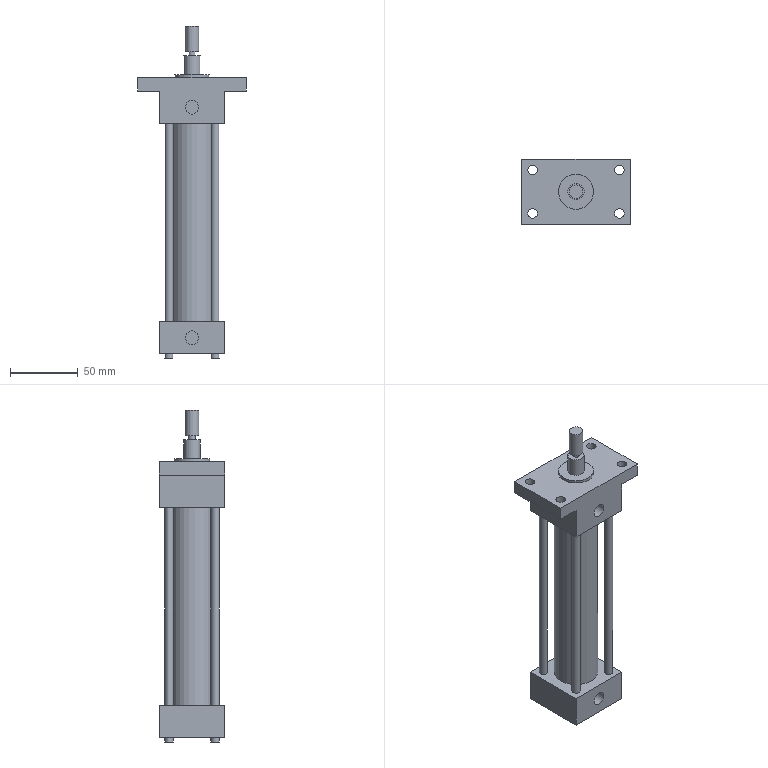Part | NX | features solid 2 | 1 solid | 48 faces | box 80 x 48 x 245 mm | volume 201071 mm3 | plane 28 | cylinder 20 | commonest cylinder face diameters 6 x8 7 x4 10 x3 5 x1 12 x1 26 x1
STEP:
#1=CARTESIAN_POINT('',(560.,11.,-204.));
#2=VERTEX_POINT('',#1);
#3=CARTESIAN_POINT('',(560.,-5.,-204.));
#4=DIRECTION('',(0.,0.,1.));
#5=DIRECTION('',(0.,1.,0.));
#6=AXIS2_PLACEMENT_3D('',#3,#4,#5);
#7=CIRCLE('',#6,16.);
#8=EDGE_CURVE('',#2,#2,#7,.T.);
#9=ORIENTED_EDGE('',*,*,#8,.F.);
#10=EDGE_LOOP('',(#9));
#11=FACE_BOUND('',#10,.T.);
#12=CARTESIAN_POINT('',(560.,11.,-350.));
#13=VERTEX_POINT('',#12);
#14=CARTESIAN_POINT('',(560.,-5.,-350.));
#15=DIRECTION('',(0.,0.,1.));
#16=DIRECTION('',(0.,1.,0.));
#17=AXIS2_PLACEMENT_3D('',#14,#15,#16);
#18=CIRCLE('',#17,16.);
#19=EDGE_CURVE('',#13,#13,#18,.F.);
#20=ORIENTED_EDGE('',*,*,#19,.F.);
#21=EDGE_LOOP('',(#20));
#22=FACE_BOUND('',#21,.T.);
#23=CARTESIAN_POINT('',(560.,-5.,-374.));
#24=DIRECTION('',(0.,0.,1.));
#25=DIRECTION('',(0.,-1.,0.));
#26=AXIS2_PLACEMENT_3D('',#23,#24,#25);
#27=CYLINDRICAL_SURFACE('',#26,16.);
#28=ADVANCED_FACE('',(#11,#22),#27,.T.);
#29=CARTESIAN_POINT('',(560.,-11.,-154.));
#30=VERTEX_POINT('',#29);
#31=CARTESIAN_POINT('',(560.,-5.,-154.));
#32=DIRECTION('',(0.,0.,-1.));
#33=DIRECTION('',(0.,-1.,0.));
#34=AXIS2_PLACEMENT_3D('',#31,#32,#33);
#35=CIRCLE('',#34,6.);
#36=EDGE_CURVE('',#30,#30,#35,.T.);
#37=ORIENTED_EDGE('',*,*,#36,.F.);
#38=EDGE_LOOP('',(#37));
#39=FACE_BOUND('',#38,.T.);
#40=CARTESIAN_POINT('',(560.,-7.5,-154.));
#41=VERTEX_POINT('',#40);
#42=CARTESIAN_POINT('',(560.,-5.,-154.));
#43=DIRECTION('',(0.,0.,-1.));
#44=DIRECTION('',(0.,-1.,0.));
#45=AXIS2_PLACEMENT_3D('',#42,#43,#44);
#46=CIRCLE('',#45,2.5);
#47=EDGE_CURVE('',#41,#41,#46,.T.);
#48=ORIENTED_EDGE('',*,*,#47,.T.);
#49=EDGE_LOOP('',(#48));
#50=FACE_BOUND('',#49,.T.);
#51=CARTESIAN_POINT('',(560.,-5.,-154.));
#52=DIRECTION('',(0.,0.,1.));
#53=DIRECTION('',(0.,-1.,0.));
#54=AXIS2_PLACEMENT_3D('',#51,#52,#53);
#55=PLANE('',#54);
#56=ADVANCED_FACE('',(#39,#50),#55,.T.);
#57=CARTESIAN_POINT('',(560.,-18.,-168.));
#58=VERTEX_POINT('',#57);
#59=CARTESIAN_POINT('',(560.,-5.,-168.));
#60=DIRECTION('',(0.,0.,-1.));
#61=DIRECTION('',(0.,-1.,0.));
#62=AXIS2_PLACEMENT_3D('',#59,#60,#61);
#63=CIRCLE('',#62,13.);
#64=EDGE_CURVE('',#58,#58,#63,.T.);
#65=ORIENTED_EDGE('',*,*,#64,.F.);
#66=EDGE_LOOP('',(#65));
#67=FACE_BOUND('',#66,.T.);
#68=CARTESIAN_POINT('',(560.,-11.,-168.));
#69=VERTEX_POINT('',#68);
#70=CARTESIAN_POINT('',(560.,-5.,-168.));
#71=DIRECTION('',(0.,0.,-1.));
#72=DIRECTION('',(0.,-1.,0.));
#73=AXIS2_PLACEMENT_3D('',#70,#71,#72);
#74=CIRCLE('',#73,6.);
#75=EDGE_CURVE('',#69,#69,#74,.F.);
#76=ORIENTED_EDGE('',*,*,#75,.F.);
#77=EDGE_LOOP('',(#76));
#78=FACE_BOUND('',#77,.T.);
#79=CARTESIAN_POINT('',(560.,-5.,-168.));
#80=DIRECTION('',(0.,0.,1.));
#81=DIRECTION('',(0.,-1.,0.));
#82=AXIS2_PLACEMENT_3D('',#79,#80,#81);
#83=PLANE('',#82);
#84=ADVANCED_FACE('',(#67,#78),#83,.T.);
#85=CARTESIAN_POINT('',(528.,7.5,-170.));
#86=VERTEX_POINT('',#85);
#87=CARTESIAN_POINT('',(528.,11.,-170.));
#88=DIRECTION('',(0.,0.,-1.));
#89=DIRECTION('',(0.,-1.,0.));
#90=AXIS2_PLACEMENT_3D('',#87,#88,#89);
#91=CIRCLE('',#90,3.5);
#92=EDGE_CURVE('',#86,#86,#91,.T.);
#93=ORIENTED_EDGE('',*,*,#92,.T.);
#94=EDGE_LOOP('',(#93));
#95=FACE_BOUND('',#94,.T.);
#96=CARTESIAN_POINT('',(592.,-24.5,-170.));
#97=VERTEX_POINT('',#96);
#98=CARTESIAN_POINT('',(592.,-21.,-170.));
#99=DIRECTION('',(0.,0.,-1.));
#100=DIRECTION('',(0.,-1.,0.));
#101=AXIS2_PLACEMENT_3D('',#98,#99,#100);
#102=CIRCLE('',#101,3.5);
#103=EDGE_CURVE('',#97,#97,#102,.T.);
#104=ORIENTED_EDGE('',*,*,#103,.T.);
#105=EDGE_LOOP('',(#104));
#106=FACE_BOUND('',#105,.T.);
#107=CARTESIAN_POINT('',(520.,19.,-170.));
#108=VERTEX_POINT('',#107);
#109=CARTESIAN_POINT('',(520.,-29.,-170.));
#110=VERTEX_POINT('',#109);
#111=CARTESIAN_POINT('',(520.,19.,-170.));
#112=DIRECTION('',(0.,-1.,0.));
#113=VECTOR('',#112,1000.);
#114=LINE('',#111,#113);
#115=EDGE_CURVE('',#108,#110,#114,.T.);
#116=ORIENTED_EDGE('',*,*,#115,.T.);
#117=CARTESIAN_POINT('',(600.,-29.,-170.));
#118=VERTEX_POINT('',#117);
#119=CARTESIAN_POINT('',(600.,-29.,-170.));
#120=DIRECTION('',(-1.,0.,0.));
#121=VECTOR('',#120,1000.);
#122=LINE('',#119,#121);
#123=EDGE_CURVE('',#118,#110,#122,.T.);
#124=ORIENTED_EDGE('',*,*,#123,.F.);
#125=CARTESIAN_POINT('',(600.,19.,-170.));
#126=VERTEX_POINT('',#125);
#127=CARTESIAN_POINT('',(600.,19.,-170.));
#128=DIRECTION('',(0.,-1.,0.));
#129=VECTOR('',#128,1000.);
#130=LINE('',#127,#129);
#131=EDGE_CURVE('',#126,#118,#130,.T.);
#132=ORIENTED_EDGE('',*,*,#131,.F.);
#133=CARTESIAN_POINT('',(536.,19.,-170.));
#134=DIRECTION('',(-1.,0.,0.));
#135=VECTOR('',#134,1000.);
#136=LINE('',#133,#135);
#137=EDGE_CURVE('',#126,#108,#136,.T.);
#138=ORIENTED_EDGE('',*,*,#137,.T.);
#139=EDGE_LOOP('',(#116,#124,#132,#138));
#140=FACE_BOUND('',#139,.T.);
#141=CARTESIAN_POINT('',(592.,7.5,-170.));
#142=VERTEX_POINT('',#141);
#143=CARTESIAN_POINT('',(592.,11.,-170.));
#144=DIRECTION('',(0.,0.,-1.));
#145=DIRECTION('',(0.,-1.,0.));
#146=AXIS2_PLACEMENT_3D('',#143,#144,#145);
#147=CIRCLE('',#146,3.5);
#148=EDGE_CURVE('',#142,#142,#147,.T.);
#149=ORIENTED_EDGE('',*,*,#148,.T.);
#150=EDGE_LOOP('',(#149));
#151=FACE_BOUND('',#150,.T.);
#152=CARTESIAN_POINT('',(528.,-24.5,-170.));
#153=VERTEX_POINT('',#152);
#154=CARTESIAN_POINT('',(528.,-21.,-170.));
#155=DIRECTION('',(0.,0.,-1.));
#156=DIRECTION('',(0.,-1.,0.));
#157=AXIS2_PLACEMENT_3D('',#154,#155,#156);
#158=CIRCLE('',#157,3.5);
#159=EDGE_CURVE('',#153,#153,#158,.T.);
#160=ORIENTED_EDGE('',*,*,#159,.T.);
#161=EDGE_LOOP('',(#160));
#162=FACE_BOUND('',#161,.T.);
#163=CARTESIAN_POINT('',(560.,8.,-170.));
#164=VERTEX_POINT('',#163);
#165=CARTESIAN_POINT('',(560.,-5.,-170.));
#166=DIRECTION('',(0.,0.,1.));
#167=DIRECTION('',(0.,1.,0.));
#168=AXIS2_PLACEMENT_3D('',#165,#166,#167);
#169=CIRCLE('',#168,13.);
#170=EDGE_CURVE('',#164,#164,#169,.F.);
#171=ORIENTED_EDGE('',*,*,#170,.T.);
#172=EDGE_LOOP('',(#171));
#173=FACE_BOUND('',#172,.T.);
#174=CARTESIAN_POINT('',(520.,-29.,-170.));
#175=DIRECTION('',(0.,0.,-1.));
#176=DIRECTION('',(0.,1.,0.));
#177=AXIS2_PLACEMENT_3D('',#174,#175,#176);
#178=PLANE('',#177);
#179=ADVANCED_FACE('',(#95,#106,#140,#151,#162,#173),#178,.F.);
#180=CARTESIAN_POINT('',(584.,-29.,-180.));
#181=VERTEX_POINT('',#180);
#182=CARTESIAN_POINT('',(584.,19.,-180.));
#183=VERTEX_POINT('',#182);
#184=CARTESIAN_POINT('',(584.,-29.,-180.));
#185=DIRECTION('',(0.,1.,0.));
#186=VECTOR('',#185,1000.);
#187=LINE('',#184,#186);
#188=EDGE_CURVE('',#181,#183,#187,.T.);
#189=ORIENTED_EDGE('',*,*,#188,.T.);
#190=CARTESIAN_POINT('',(600.,19.,-180.));
#191=VERTEX_POINT('',#190);
#192=CARTESIAN_POINT('',(536.,19.,-180.));
#193=DIRECTION('',(-1.,0.,0.));
#194=VECTOR('',#193,1000.);
#195=LINE('',#192,#194);
#196=EDGE_CURVE('',#191,#183,#195,.T.);
#197=ORIENTED_EDGE('',*,*,#196,.F.);
#198=CARTESIAN_POINT('',(600.,-29.,-180.));
#199=VERTEX_POINT('',#198);
#200=CARTESIAN_POINT('',(600.,19.,-180.));
#201=DIRECTION('',(0.,-1.,0.));
#202=VECTOR('',#201,1000.);
#203=LINE('',#200,#202);
#204=EDGE_CURVE('',#191,#199,#203,.T.);
#205=ORIENTED_EDGE('',*,*,#204,.T.);
#206=CARTESIAN_POINT('',(600.,-29.,-180.));
#207=DIRECTION('',(-1.,0.,0.));
#208=VECTOR('',#207,1000.);
#209=LINE('',#206,#208);
#210=EDGE_CURVE('',#199,#181,#209,.T.);
#211=ORIENTED_EDGE('',*,*,#210,.T.);
#212=EDGE_LOOP('',(#189,#197,#205,#211));
#213=FACE_BOUND('',#212,.T.);
#214=CARTESIAN_POINT('',(592.,-24.5,-180.));
#215=VERTEX_POINT('',#214);
#216=CARTESIAN_POINT('',(592.,-21.,-180.));
#217=DIRECTION('',(0.,0.,-1.));
#218=DIRECTION('',(0.,-1.,0.));
#219=AXIS2_PLACEMENT_3D('',#216,#217,#218);
#220=CIRCLE('',#219,3.5);
#221=EDGE_CURVE('',#215,#215,#220,.T.);
#222=ORIENTED_EDGE('',*,*,#221,.F.);
#223=EDGE_LOOP('',(#222));
#224=FACE_BOUND('',#223,.T.);
#225=CARTESIAN_POINT('',(592.,7.5,-180.));
#226=VERTEX_POINT('',#225);
#227=CARTESIAN_POINT('',(592.,11.,-180.));
#228=DIRECTION('',(0.,0.,-1.));
#229=DIRECTION('',(0.,-1.,0.));
#230=AXIS2_PLACEMENT_3D('',#227,#228,#229);
#231=CIRCLE('',#230,3.5);
#232=EDGE_CURVE('',#226,#226,#231,.T.);
#233=ORIENTED_EDGE('',*,*,#232,.F.);
#234=EDGE_LOOP('',(#233));
#235=FACE_BOUND('',#234,.T.);
#236=CARTESIAN_POINT('',(520.,-29.,-180.));
#237=DIRECTION('',(0.,0.,-1.));
#238=DIRECTION('',(0.,1.,0.));
#239=AXIS2_PLACEMENT_3D('',#236,#237,#238);
#240=PLANE('',#239);
#241=ADVANCED_FACE('',(#213,#224,#235),#240,.T.);
#242=ORIENTED_EDGE('',*,*,#115,.F.);
#243=CARTESIAN_POINT('',(520.,19.,-180.));
#244=VERTEX_POINT('',#243);
#245=CARTESIAN_POINT('',(520.,19.,-180.));
#246=DIRECTION('',(0.,0.,1.));
#247=VECTOR('',#246,1000.);
#248=LINE('',#245,#247);
#249=EDGE_CURVE('',#244,#108,#248,.T.);
#250=ORIENTED_EDGE('',*,*,#249,.F.);
#251=CARTESIAN_POINT('',(520.,-29.,-180.));
#252=VERTEX_POINT('',#251);
#253=CARTESIAN_POINT('',(520.,19.,-180.));
#254=DIRECTION('',(0.,-1.,0.));
#255=VECTOR('',#254,1000.);
#256=LINE('',#253,#255);
#257=EDGE_CURVE('',#244,#252,#256,.T.);
#258=ORIENTED_EDGE('',*,*,#257,.T.);
#259=CARTESIAN_POINT('',(520.,-29.,-180.));
#260=DIRECTION('',(0.,0.,1.));
#261=VECTOR('',#260,1000.);
#262=LINE('',#259,#261);
#263=EDGE_CURVE('',#252,#110,#262,.T.);
#264=ORIENTED_EDGE('',*,*,#263,.T.);
#265=EDGE_LOOP('',(#242,#250,#258,#264));
#266=FACE_BOUND('',#265,.T.);
#267=CARTESIAN_POINT('',(520.,19.,-180.));
#268=DIRECTION('',(1.,0.,0.));
#269=DIRECTION('',(0.,0.,-1.));
#270=AXIS2_PLACEMENT_3D('',#267,#268,#269);
#271=PLANE('',#270);
#272=ADVANCED_FACE('',(#266),#271,.F.);
#273=CARTESIAN_POINT('',(565.,-29.,-192.));
#274=VERTEX_POINT('',#273);
#275=CARTESIAN_POINT('',(560.,-29.,-192.));
#276=DIRECTION('',(0.,-1.,0.));
#277=DIRECTION('',(1.,0.,0.));
#278=AXIS2_PLACEMENT_3D('',#275,#276,#277);
#279=CIRCLE('',#278,5.);
#280=EDGE_CURVE('',#274,#274,#279,.T.);
#281=ORIENTED_EDGE('',*,*,#280,.F.);
#282=EDGE_LOOP('',(#281));
#283=FACE_BOUND('',#282,.T.);
#284=ORIENTED_EDGE('',*,*,#123,.T.);
#285=ORIENTED_EDGE('',*,*,#263,.F.);
#286=CARTESIAN_POINT('',(536.,-29.,-180.));
#287=VERTEX_POINT('',#286);
#288=CARTESIAN_POINT('',(600.,-29.,-180.));
#289=DIRECTION('',(-1.,0.,0.));
#290=VECTOR('',#289,1000.);
#291=LINE('',#288,#290);
#292=EDGE_CURVE('',#287,#252,#291,.T.);
#293=ORIENTED_EDGE('',*,*,#292,.F.);
#294=CARTESIAN_POINT('',(536.,-29.,-204.));
#295=VERTEX_POINT('',#294);
#296=CARTESIAN_POINT('',(536.,-29.,-204.));
#297=DIRECTION('',(0.,0.,1.));
#298=VECTOR('',#297,1000.);
#299=LINE('',#296,#298);
#300=EDGE_CURVE('',#295,#287,#299,.T.);
#301=ORIENTED_EDGE('',*,*,#300,.F.);
#302=CARTESIAN_POINT('',(584.,-29.,-204.));
#303=VERTEX_POINT('',#302);
#304=CARTESIAN_POINT('',(536.,-29.,-204.));
#305=DIRECTION('',(1.,0.,0.));
#306=VECTOR('',#305,1000.);
#307=LINE('',#304,#306);
#308=EDGE_CURVE('',#295,#303,#307,.T.);
#309=ORIENTED_EDGE('',*,*,#308,.T.);
#310=CARTESIAN_POINT('',(584.,-29.,-204.));
#311=DIRECTION('',(0.,0.,1.));
#312=VECTOR('',#311,1000.);
#313=LINE('',#310,#312);
#314=EDGE_CURVE('',#303,#181,#313,.T.);
#315=ORIENTED_EDGE('',*,*,#314,.T.);
#316=ORIENTED_EDGE('',*,*,#210,.F.);
#317=CARTESIAN_POINT('',(600.,-29.,-180.));
#318=DIRECTION('',(0.,0.,1.));
#319=VECTOR('',#318,1000.);
#320=LINE('',#317,#319);
#321=EDGE_CURVE('',#199,#118,#320,.T.);
#322=ORIENTED_EDGE('',*,*,#321,.T.);
#323=EDGE_LOOP('',(#284,#285,#293,#301,#309,#315,#316,#322));
#324=FACE_BOUND('',#323,.T.);
#325=CARTESIAN_POINT('',(600.,-29.,-180.));
#326=DIRECTION('',(0.,-1.,0.));
#327=DIRECTION('',(0.,0.,-1.));
#328=AXIS2_PLACEMENT_3D('',#325,#326,#327);
#329=PLANE('',#328);
#330=ADVANCED_FACE('',(#283,#324),#329,.T.);
#331=ORIENTED_EDGE('',*,*,#131,.T.);
#332=ORIENTED_EDGE('',*,*,#321,.F.);
#333=ORIENTED_EDGE('',*,*,#204,.F.);
#334=CARTESIAN_POINT('',(600.,19.,-180.));
#335=DIRECTION('',(0.,0.,1.));
#336=VECTOR('',#335,1000.);
#337=LINE('',#334,#336);
#338=EDGE_CURVE('',#191,#126,#337,.T.);
#339=ORIENTED_EDGE('',*,*,#338,.T.);
#340=EDGE_LOOP('',(#331,#332,#333,#339));
#341=FACE_BOUND('',#340,.T.);
#342=CARTESIAN_POINT('',(600.,19.,-180.));
#343=DIRECTION('',(1.,0.,0.));
#344=DIRECTION('',(0.,0.,-1.));
#345=AXIS2_PLACEMENT_3D('',#342,#343,#344);
#346=PLANE('',#345);
#347=ADVANCED_FACE('',(#341),#346,.T.);
#348=ORIENTED_EDGE('',*,*,#221,.T.);
#349=EDGE_LOOP('',(#348));
#350=FACE_BOUND('',#349,.T.);
#351=ORIENTED_EDGE('',*,*,#103,.F.);
#352=EDGE_LOOP('',(#351));
#353=FACE_BOUND('',#352,.T.);
#354=CARTESIAN_POINT('',(592.,-21.,-180.));
#355=DIRECTION('',(0.,0.,1.));
#356=DIRECTION('',(0.,-1.,0.));
#357=AXIS2_PLACEMENT_3D('',#354,#355,#356);
#358=CYLINDRICAL_SURFACE('',#357,3.5);
#359=ADVANCED_FACE('',(#350,#353),#358,.F.);
#360=ORIENTED_EDGE('',*,*,#137,.F.);
#361=ORIENTED_EDGE('',*,*,#338,.F.);
#362=ORIENTED_EDGE('',*,*,#196,.T.);
#363=CARTESIAN_POINT('',(584.,19.,-204.));
#364=VERTEX_POINT('',#363);
#365=CARTESIAN_POINT('',(584.,19.,-204.));
#366=DIRECTION('',(0.,0.,1.));
#367=VECTOR('',#366,1000.);
#368=LINE('',#365,#367);
#369=EDGE_CURVE('',#364,#183,#368,.T.);
#370=ORIENTED_EDGE('',*,*,#369,.F.);
#371=CARTESIAN_POINT('',(536.,19.,-204.));
#372=VERTEX_POINT('',#371);
#373=CARTESIAN_POINT('',(584.,19.,-204.));
#374=DIRECTION('',(-1.,0.,0.));
#375=VECTOR('',#374,1000.);
#376=LINE('',#373,#375);
#377=EDGE_CURVE('',#364,#372,#376,.T.);
#378=ORIENTED_EDGE('',*,*,#377,.T.);
#379=CARTESIAN_POINT('',(536.,19.,-180.));
#380=VERTEX_POINT('',#379);
#381=CARTESIAN_POINT('',(536.,19.,-204.));
#382=DIRECTION('',(0.,0.,1.));
#383=VECTOR('',#382,1000.);
#384=LINE('',#381,#383);
#385=EDGE_CURVE('',#372,#380,#384,.T.);
#386=ORIENTED_EDGE('',*,*,#385,.T.);
#387=CARTESIAN_POINT('',(536.,19.,-180.));
#388=DIRECTION('',(-1.,0.,0.));
#389=VECTOR('',#388,1000.);
#390=LINE('',#387,#389);
#391=EDGE_CURVE('',#380,#244,#390,.T.);
#392=ORIENTED_EDGE('',*,*,#391,.T.);
#393=ORIENTED_EDGE('',*,*,#249,.T.);
#394=EDGE_LOOP('',(#360,#361,#362,#370,#378,#386,#392,#393));
#395=FACE_BOUND('',#394,.T.);
#396=CARTESIAN_POINT('',(536.,19.,-180.));
#397=DIRECTION('',(0.,-1.,0.));
#398=DIRECTION('',(-1.,0.,0.));
#399=AXIS2_PLACEMENT_3D('',#396,#397,#398);
#400=PLANE('',#399);
#401=ADVANCED_FACE('',(#395),#400,.F.);
#402=ORIENTED_EDGE('',*,*,#232,.T.);
#403=EDGE_LOOP('',(#402));
#404=FACE_BOUND('',#403,.T.);
#405=ORIENTED_EDGE('',*,*,#148,.F.);
#406=EDGE_LOOP('',(#405));
#407=FACE_BOUND('',#406,.T.);
#408=CARTESIAN_POINT('',(592.,11.,-180.));
#409=DIRECTION('',(0.,0.,1.));
#410=DIRECTION('',(0.,-1.,0.));
#411=AXIS2_PLACEMENT_3D('',#408,#409,#410);
#412=CYLINDRICAL_SURFACE('',#411,3.5);
#413=ADVANCED_FACE('',(#404,#407),#412,.F.);
#414=CARTESIAN_POINT('',(528.,-24.5,-180.));
#415=VERTEX_POINT('',#414);
#416=CARTESIAN_POINT('',(528.,-21.,-180.));
#417=DIRECTION('',(0.,0.,-1.));
#418=DIRECTION('',(0.,-1.,0.));
#419=AXIS2_PLACEMENT_3D('',#416,#417,#418);
#420=CIRCLE('',#419,3.5);
#421=EDGE_CURVE('',#415,#415,#420,.T.);
#422=ORIENTED_EDGE('',*,*,#421,.T.);
#423=EDGE_LOOP('',(#422));
#424=FACE_BOUND('',#423,.T.);
#425=ORIENTED_EDGE('',*,*,#159,.F.);
#426=EDGE_LOOP('',(#425));
#427=FACE_BOUND('',#426,.T.);
#428=CARTESIAN_POINT('',(528.,-21.,-180.));
#429=DIRECTION('',(0.,0.,1.));
#430=DIRECTION('',(0.,-1.,0.));
#431=AXIS2_PLACEMENT_3D('',#428,#429,#430);
#432=CYLINDRICAL_SURFACE('',#431,3.5);
#433=ADVANCED_FACE('',(#424,#427),#432,.F.);
#434=CARTESIAN_POINT('',(528.,7.5,-180.));
#435=VERTEX_POINT('',#434);
#436=CARTESIAN_POINT('',(528.,11.,-180.));
#437=DIRECTION('',(0.,0.,-1.));
#438=DIRECTION('',(0.,-1.,0.));
#439=AXIS2_PLACEMENT_3D('',#436,#437,#438);
#440=CIRCLE('',#439,3.5);
#441=EDGE_CURVE('',#435,#435,#440,.T.);
#442=ORIENTED_EDGE('',*,*,#441,.T.);
#443=EDGE_LOOP('',(#442));
#444=FACE_BOUND('',#443,.T.);
#445=ORIENTED_EDGE('',*,*,#92,.F.);
#446=EDGE_LOOP('',(#445));
#447=FACE_BOUND('',#446,.T.);
#448=CARTESIAN_POINT('',(528.,11.,-180.));
#449=DIRECTION('',(0.,0.,1.));
#450=DIRECTION('',(0.,-1.,0.));
#451=AXIS2_PLACEMENT_3D('',#448,#449,#450);
#452=CYLINDRICAL_SURFACE('',#451,3.5);
#453=ADVANCED_FACE('',(#444,#447),#452,.F.);
#454=CARTESIAN_POINT('',(536.,19.,-180.));
#455=DIRECTION('',(0.,-1.,0.));
#456=VECTOR('',#455,1000.);
#457=LINE('',#454,#456);
#458=EDGE_CURVE('',#380,#287,#457,.T.);
#459=ORIENTED_EDGE('',*,*,#458,.T.);
#460=ORIENTED_EDGE('',*,*,#292,.T.);
#461=ORIENTED_EDGE('',*,*,#257,.F.);
#462=ORIENTED_EDGE('',*,*,#391,.F.);
#463=EDGE_LOOP('',(#459,#460,#461,#462));
#464=FACE_BOUND('',#463,.T.);
#465=ORIENTED_EDGE('',*,*,#421,.F.);
#466=EDGE_LOOP('',(#465));
#467=FACE_BOUND('',#466,.T.);
#468=ORIENTED_EDGE('',*,*,#441,.F.);
#469=EDGE_LOOP('',(#468));
#470=FACE_BOUND('',#469,.T.);
#471=CARTESIAN_POINT('',(520.,-29.,-180.));
#472=DIRECTION('',(0.,0.,-1.));
#473=DIRECTION('',(0.,1.,0.));
#474=AXIS2_PLACEMENT_3D('',#471,#472,#473);
#475=PLANE('',#474);
#476=ADVANCED_FACE('',(#464,#467,#470),#475,.T.);
#477=ORIENTED_EDGE('',*,*,#458,.F.);
#478=ORIENTED_EDGE('',*,*,#385,.F.);
#479=CARTESIAN_POINT('',(536.,19.,-204.));
#480=DIRECTION('',(0.,-1.,0.));
#481=VECTOR('',#480,1000.);
#482=LINE('',#479,#481);
#483=EDGE_CURVE('',#372,#295,#482,.T.);
#484=ORIENTED_EDGE('',*,*,#483,.T.);
#485=ORIENTED_EDGE('',*,*,#300,.T.);
#486=EDGE_LOOP('',(#477,#478,#484,#485));
#487=FACE_BOUND('',#486,.T.);
#488=CARTESIAN_POINT('',(536.,19.,-204.));
#489=DIRECTION('',(1.,0.,0.));
#490=DIRECTION('',(0.,0.,-1.));
#491=AXIS2_PLACEMENT_3D('',#488,#489,#490);
#492=PLANE('',#491);
#493=ADVANCED_FACE('',(#487),#492,.F.);
#494=ORIENTED_EDGE('',*,*,#188,.F.);
#495=ORIENTED_EDGE('',*,*,#314,.F.);
#496=CARTESIAN_POINT('',(584.,-29.,-204.));
#497=DIRECTION('',(0.,1.,0.));
#498=VECTOR('',#497,1000.);
#499=LINE('',#496,#498);
#500=EDGE_CURVE('',#303,#364,#499,.T.);
#501=ORIENTED_EDGE('',*,*,#500,.T.);
#502=ORIENTED_EDGE('',*,*,#369,.T.);
#503=EDGE_LOOP('',(#494,#495,#501,#502));
#504=FACE_BOUND('',#503,.T.);
#505=CARTESIAN_POINT('',(584.,-29.,-204.));
#506=DIRECTION('',(-1.,0.,0.));
#507=DIRECTION('',(0.,0.,1.));
#508=AXIS2_PLACEMENT_3D('',#505,#506,#507);
#509=PLANE('',#508);
#510=ADVANCED_FACE('',(#504),#509,.F.);
#511=CARTESIAN_POINT('',(543.,-19.,-204.));
#512=VERTEX_POINT('',#511);
#513=CARTESIAN_POINT('',(543.,-22.,-204.));
#514=DIRECTION('',(0.,0.,1.));
#515=DIRECTION('',(0.,1.,0.));
#516=AXIS2_PLACEMENT_3D('',#513,#514,#515);
#517=CIRCLE('',#516,3.);
#518=EDGE_CURVE('',#512,#512,#517,.T.);
#519=ORIENTED_EDGE('',*,*,#518,.T.);
#520=EDGE_LOOP('',(#519));
#521=FACE_BOUND('',#520,.T.);
#522=CARTESIAN_POINT('',(543.,15.,-204.));
#523=VERTEX_POINT('',#522);
#524=CARTESIAN_POINT('',(543.,12.,-204.));
#525=DIRECTION('',(0.,0.,1.));
#526=DIRECTION('',(0.,1.,0.));
#527=AXIS2_PLACEMENT_3D('',#524,#525,#526);
#528=CIRCLE('',#527,3.);
#529=EDGE_CURVE('',#523,#523,#528,.T.);
#530=ORIENTED_EDGE('',*,*,#529,.T.);
#531=EDGE_LOOP('',(#530));
#532=FACE_BOUND('',#531,.T.);
#533=CARTESIAN_POINT('',(577.,15.,-204.));
#534=VERTEX_POINT('',#533);
#535=CARTESIAN_POINT('',(577.,12.,-204.));
#536=DIRECTION('',(0.,0.,1.));
#537=DIRECTION('',(0.,1.,0.));
#538=AXIS2_PLACEMENT_3D('',#535,#536,#537);
#539=CIRCLE('',#538,3.);
#540=EDGE_CURVE('',#534,#534,#539,.T.);
#541=ORIENTED_EDGE('',*,*,#540,.T.);
#542=EDGE_LOOP('',(#541));
#543=FACE_BOUND('',#542,.T.);
#544=CARTESIAN_POINT('',(577.,-19.,-204.));
#545=VERTEX_POINT('',#544);
#546=CARTESIAN_POINT('',(577.,-22.,-204.));
#547=DIRECTION('',(0.,0.,1.));
#548=DIRECTION('',(0.,1.,0.));
#549=AXIS2_PLACEMENT_3D('',#546,#547,#548);
#550=CIRCLE('',#549,3.);
#551=EDGE_CURVE('',#545,#545,#550,.T.);
#552=ORIENTED_EDGE('',*,*,#551,.T.);
#553=EDGE_LOOP('',(#552));
#554=FACE_BOUND('',#553,.T.);
#555=ORIENTED_EDGE('',*,*,#8,.T.);
#556=EDGE_LOOP('',(#555));
#557=FACE_BOUND('',#556,.T.);
#558=ORIENTED_EDGE('',*,*,#377,.F.);
#559=ORIENTED_EDGE('',*,*,#500,.F.);
#560=ORIENTED_EDGE('',*,*,#308,.F.);
#561=ORIENTED_EDGE('',*,*,#483,.F.);
#562=EDGE_LOOP('',(#558,#559,#560,#561));
#563=FACE_BOUND('',#562,.T.);
#564=CARTESIAN_POINT('',(536.,19.,-204.));
#565=DIRECTION('',(0.,0.,-1.));
#566=DIRECTION('',(0.,1.,0.));
#567=AXIS2_PLACEMENT_3D('',#564,#565,#566);
#568=PLANE('',#567);
#569=ADVANCED_FACE('',(#521,#532,#543,#554,#557,#563),#568,.T.);
#570=ORIENTED_EDGE('',*,*,#64,.T.);
#571=EDGE_LOOP('',(#570));
#572=FACE_BOUND('',#571,.T.);
#573=ORIENTED_EDGE('',*,*,#170,.F.);
#574=EDGE_LOOP('',(#573));
#575=FACE_BOUND('',#574,.T.);
#576=CARTESIAN_POINT('',(560.,-5.,-168.));
#577=DIRECTION('',(0.,0.,-1.));
#578=DIRECTION('',(0.,1.,0.));
#579=AXIS2_PLACEMENT_3D('',#576,#577,#578);
#580=CYLINDRICAL_SURFACE('',#579,13.);
#581=ADVANCED_FACE('',(#572,#575),#580,.T.);
#582=ORIENTED_EDGE('',*,*,#75,.T.);
#583=EDGE_LOOP('',(#582));
#584=FACE_BOUND('',#583,.T.);
#585=ORIENTED_EDGE('',*,*,#36,.T.);
#586=EDGE_LOOP('',(#585));
#587=FACE_BOUND('',#586,.T.);
#588=CARTESIAN_POINT('',(560.,-5.,-154.));
#589=DIRECTION('',(0.,0.,-1.));
#590=DIRECTION('',(0.,1.,0.));
#591=AXIS2_PLACEMENT_3D('',#588,#589,#590);
#592=CYLINDRICAL_SURFACE('',#591,6.);
#593=ADVANCED_FACE('',(#584,#587),#592,.T.);
#594=CARTESIAN_POINT('',(584.,19.,-350.));
#595=VERTEX_POINT('',#594);
#596=CARTESIAN_POINT('',(536.,19.,-350.));
#597=VERTEX_POINT('',#596);
#598=CARTESIAN_POINT('',(584.,19.,-350.));
#599=DIRECTION('',(-1.,0.,0.));
#600=VECTOR('',#599,1000.);
#601=LINE('',#598,#600);
#602=EDGE_CURVE('',#595,#597,#601,.T.);
#603=ORIENTED_EDGE('',*,*,#602,.F.);
#604=CARTESIAN_POINT('',(584.,19.,-374.));
#605=VERTEX_POINT('',#604);
#606=CARTESIAN_POINT('',(584.,19.,-374.));
#607=DIRECTION('',(0.,0.,1.));
#608=VECTOR('',#607,1000.);
#609=LINE('',#606,#608);
#610=EDGE_CURVE('',#605,#595,#609,.T.);
#611=ORIENTED_EDGE('',*,*,#610,.F.);
#612=CARTESIAN_POINT('',(536.,19.,-374.));
#613=VERTEX_POINT('',#612);
#614=CARTESIAN_POINT('',(584.,19.,-374.));
#615=DIRECTION('',(-1.,0.,0.));
#616=VECTOR('',#615,1000.);
#617=LINE('',#614,#616);
#618=EDGE_CURVE('',#605,#613,#617,.T.);
#619=ORIENTED_EDGE('',*,*,#618,.T.);
#620=CARTESIAN_POINT('',(536.,19.,-374.));
#621=DIRECTION('',(0.,0.,1.));
#622=VECTOR('',#621,1000.);
#623=LINE('',#620,#622);
#624=EDGE_CURVE('',#613,#597,#623,.T.);
#625=ORIENTED_EDGE('',*,*,#624,.T.);
#626=EDGE_LOOP('',(#603,#611,#619,#625));
#627=FACE_BOUND('',#626,.T.);
#628=CARTESIAN_POINT('',(584.,19.,-374.));
#629=DIRECTION('',(0.,-1.,0.));
#630=DIRECTION('',(-1.,0.,0.));
#631=AXIS2_PLACEMENT_3D('',#628,#629,#630);
#632=PLANE('',#631);
#633=ADVANCED_FACE('',(#627),#632,.F.);
#634=CARTESIAN_POINT('',(536.,-29.,-350.));
#635=VERTEX_POINT('',#634);
#636=CARTESIAN_POINT('',(536.,19.,-350.));
#637=DIRECTION('',(0.,-1.,0.));
#638=VECTOR('',#637,1000.);
#639=LINE('',#636,#638);
#640=EDGE_CURVE('',#597,#635,#639,.T.);
#641=ORIENTED_EDGE('',*,*,#640,.F.);
#642=ORIENTED_EDGE('',*,*,#624,.F.);
#643=CARTESIAN_POINT('',(536.,-29.,-374.));
#644=VERTEX_POINT('',#643);
#645=CARTESIAN_POINT('',(536.,19.,-374.));
#646=DIRECTION('',(0.,-1.,0.));
#647=VECTOR('',#646,1000.);
#648=LINE('',#645,#647);
#649=EDGE_CURVE('',#613,#644,#648,.T.);
#650=ORIENTED_EDGE('',*,*,#649,.T.);
#651=CARTESIAN_POINT('',(536.,-29.,-374.));
#652=DIRECTION('',(0.,0.,1.));
#653=VECTOR('',#652,1000.);
#654=LINE('',#651,#653);
#655=EDGE_CURVE('',#644,#635,#654,.T.);
#656=ORIENTED_EDGE('',*,*,#655,.T.);
#657=EDGE_LOOP('',(#641,#642,#650,#656));
#658=FACE_BOUND('',#657,.T.);
#659=CARTESIAN_POINT('',(536.,19.,-374.));
#660=DIRECTION('',(1.,0.,0.));
#661=DIRECTION('',(0.,0.,-1.));
#662=AXIS2_PLACEMENT_3D('',#659,#660,#661);
#663=PLANE('',#662);
#664=ADVANCED_FACE('',(#658),#663,.F.);
#665=CARTESIAN_POINT('',(565.,-29.,-362.));
#666=VERTEX_POINT('',#665);
#667=CARTESIAN_POINT('',(560.,-29.,-362.));
#668=DIRECTION('',(0.,-1.,0.));
#669=DIRECTION('',(1.,0.,0.));
#670=AXIS2_PLACEMENT_3D('',#667,#668,#669);
#671=CIRCLE('',#670,5.);
#672=EDGE_CURVE('',#666,#666,#671,.T.);
#673=ORIENTED_EDGE('',*,*,#672,.F.);
#674=EDGE_LOOP('',(#673));
#675=FACE_BOUND('',#674,.T.);
#676=CARTESIAN_POINT('',(584.,-29.,-350.));
#677=VERTEX_POINT('',#676);
#678=CARTESIAN_POINT('',(536.,-29.,-350.));
#679=DIRECTION('',(1.,0.,0.));
#680=VECTOR('',#679,1000.);
#681=LINE('',#678,#680);
#682=EDGE_CURVE('',#635,#677,#681,.T.);
#683=ORIENTED_EDGE('',*,*,#682,.F.);
#684=ORIENTED_EDGE('',*,*,#655,.F.);
#685=CARTESIAN_POINT('',(584.,-29.,-374.));
#686=VERTEX_POINT('',#685);
#687=CARTESIAN_POINT('',(536.,-29.,-374.));
#688=DIRECTION('',(1.,0.,0.));
#689=VECTOR('',#688,1000.);
#690=LINE('',#687,#689);
#691=EDGE_CURVE('',#644,#686,#690,.T.);
#692=ORIENTED_EDGE('',*,*,#691,.T.);
#693=CARTESIAN_POINT('',(584.,-29.,-374.));
#694=DIRECTION('',(0.,0.,1.));
#695=VECTOR('',#694,1000.);
#696=LINE('',#693,#695);
#697=EDGE_CURVE('',#686,#677,#696,.T.);
#698=ORIENTED_EDGE('',*,*,#697,.T.);
#699=EDGE_LOOP('',(#683,#684,#692,#698));
#700=FACE_BOUND('',#699,.T.);
#701=CARTESIAN_POINT('',(536.,-29.,-374.));
#702=DIRECTION('',(0.,1.,0.));
#703=DIRECTION('',(1.,0.,0.));
#704=AXIS2_PLACEMENT_3D('',#701,#702,#703);
#705=PLANE('',#704);
#706=ADVANCED_FACE('',(#675,#700),#705,.F.);
#707=CARTESIAN_POINT('',(584.,-29.,-350.));
#708=DIRECTION('',(0.,1.,0.));
#709=VECTOR('',#708,1000.);
#710=LINE('',#707,#709);
#711=EDGE_CURVE('',#677,#595,#710,.T.);
#712=ORIENTED_EDGE('',*,*,#711,.F.);
#713=ORIENTED_EDGE('',*,*,#697,.F.);
#714=CARTESIAN_POINT('',(584.,-29.,-374.));
#715=DIRECTION('',(0.,1.,0.));
#716=VECTOR('',#715,1000.);
#717=LINE('',#714,#716);
#718=EDGE_CURVE('',#686,#605,#717,.T.);
#719=ORIENTED_EDGE('',*,*,#718,.T.);
#720=ORIENTED_EDGE('',*,*,#610,.T.);
#721=EDGE_LOOP('',(#712,#713,#719,#720));
#722=FACE_BOUND('',#721,.T.);
#723=CARTESIAN_POINT('',(584.,-29.,-374.));
#724=DIRECTION('',(-1.,0.,0.));
#725=DIRECTION('',(0.,0.,1.));
#726=AXIS2_PLACEMENT_3D('',#723,#724,#725);
#727=PLANE('',#726);
#728=ADVANCED_FACE('',(#722),#727,.F.);
#729=CARTESIAN_POINT('',(543.,-19.,-350.));
#730=VERTEX_POINT('',#729);
#731=CARTESIAN_POINT('',(543.,-22.,-350.));
#732=DIRECTION('',(0.,0.,1.));
#733=DIRECTION('',(0.,1.,0.));
#734=AXIS2_PLACEMENT_3D('',#731,#732,#733);
#735=CIRCLE('',#734,3.);
#736=EDGE_CURVE('',#730,#730,#735,.T.);
#737=ORIENTED_EDGE('',*,*,#736,.F.);
#738=EDGE_LOOP('',(#737));
#739=FACE_BOUND('',#738,.T.);
#740=CARTESIAN_POINT('',(543.,15.,-350.));
#741=VERTEX_POINT('',#740);
#742=CARTESIAN_POINT('',(543.,12.,-350.));
#743=DIRECTION('',(0.,0.,1.));
#744=DIRECTION('',(0.,1.,0.));
#745=AXIS2_PLACEMENT_3D('',#742,#743,#744);
#746=CIRCLE('',#745,3.);
#747=EDGE_CURVE('',#741,#741,#746,.T.);
#748=ORIENTED_EDGE('',*,*,#747,.F.);
#749=EDGE_LOOP('',(#748));
#750=FACE_BOUND('',#749,.T.);
#751=CARTESIAN_POINT('',(577.,15.,-350.));
#752=VERTEX_POINT('',#751);
#753=CARTESIAN_POINT('',(577.,12.,-350.));
#754=DIRECTION('',(0.,0.,1.));
#755=DIRECTION('',(0.,1.,0.));
#756=AXIS2_PLACEMENT_3D('',#753,#754,#755);
#757=CIRCLE('',#756,3.);
#758=EDGE_CURVE('',#752,#752,#757,.T.);
#759=ORIENTED_EDGE('',*,*,#758,.F.);
#760=EDGE_LOOP('',(#759));
#761=FACE_BOUND('',#760,.T.);
#762=CARTESIAN_POINT('',(577.,-19.,-350.));
#763=VERTEX_POINT('',#762);
#764=CARTESIAN_POINT('',(577.,-22.,-350.));
#765=DIRECTION('',(0.,0.,1.));
#766=DIRECTION('',(0.,1.,0.));
#767=AXIS2_PLACEMENT_3D('',#764,#765,#766);
#768=CIRCLE('',#767,3.);
#769=EDGE_CURVE('',#763,#763,#768,.T.);
#770=ORIENTED_EDGE('',*,*,#769,.F.);
#771=EDGE_LOOP('',(#770));
#772=FACE_BOUND('',#771,.T.);
#773=ORIENTED_EDGE('',*,*,#19,.T.);
#774=EDGE_LOOP('',(#773));
#775=FACE_BOUND('',#774,.T.);
#776=ORIENTED_EDGE('',*,*,#602,.T.);
#777=ORIENTED_EDGE('',*,*,#640,.T.);
#778=ORIENTED_EDGE('',*,*,#682,.T.);
#779=ORIENTED_EDGE('',*,*,#711,.T.);
#780=EDGE_LOOP('',(#776,#777,#778,#779));
#781=FACE_BOUND('',#780,.T.);
#782=CARTESIAN_POINT('',(536.,19.,-350.));
#783=DIRECTION('',(0.,0.,-1.));
#784=DIRECTION('',(0.,1.,0.));
#785=AXIS2_PLACEMENT_3D('',#782,#783,#784);
#786=PLANE('',#785);
#787=ADVANCED_FACE('',(#739,#750,#761,#772,#775,#781),#786,.F.);
#788=CARTESIAN_POINT('',(543.,-25.,-374.));
#789=VERTEX_POINT('',#788);
#790=CARTESIAN_POINT('',(543.,-22.,-374.));
#791=DIRECTION('',(0.,0.,-1.));
#792=DIRECTION('',(0.,-1.,0.));
#793=AXIS2_PLACEMENT_3D('',#790,#791,#792);
#794=CIRCLE('',#793,3.);
#795=EDGE_CURVE('',#789,#789,#794,.T.);
#796=ORIENTED_EDGE('',*,*,#795,.F.);
#797=EDGE_LOOP('',(#796));
#798=FACE_BOUND('',#797,.T.);
#799=CARTESIAN_POINT('',(543.,9.,-374.));
#800=VERTEX_POINT('',#799);
#801=CARTESIAN_POINT('',(543.,12.,-374.));
#802=DIRECTION('',(0.,0.,-1.));
#803=DIRECTION('',(0.,-1.,0.));
#804=AXIS2_PLACEMENT_3D('',#801,#802,#803);
#805=CIRCLE('',#804,3.);
#806=EDGE_CURVE('',#800,#800,#805,.T.);
#807=ORIENTED_EDGE('',*,*,#806,.F.);
#808=EDGE_LOOP('',(#807));
#809=FACE_BOUND('',#808,.T.);
#810=CARTESIAN_POINT('',(577.,9.,-374.));
#811=VERTEX_POINT('',#810);
#812=CARTESIAN_POINT('',(577.,12.,-374.));
#813=DIRECTION('',(0.,0.,-1.));
#814=DIRECTION('',(0.,-1.,0.));
#815=AXIS2_PLACEMENT_3D('',#812,#813,#814);
#816=CIRCLE('',#815,3.);
#817=EDGE_CURVE('',#811,#811,#816,.T.);
#818=ORIENTED_EDGE('',*,*,#817,.F.);
#819=EDGE_LOOP('',(#818));
#820=FACE_BOUND('',#819,.T.);
#821=CARTESIAN_POINT('',(577.,-25.,-374.));
#822=VERTEX_POINT('',#821);
#823=CARTESIAN_POINT('',(577.,-22.,-374.));
#824=DIRECTION('',(0.,0.,-1.));
#825=DIRECTION('',(0.,-1.,0.));
#826=AXIS2_PLACEMENT_3D('',#823,#824,#825);
#827=CIRCLE('',#826,3.);
#828=EDGE_CURVE('',#822,#822,#827,.T.);
#829=ORIENTED_EDGE('',*,*,#828,.F.);
#830=EDGE_LOOP('',(#829));
#831=FACE_BOUND('',#830,.T.);
#832=ORIENTED_EDGE('',*,*,#618,.F.);
#833=ORIENTED_EDGE('',*,*,#718,.F.);
#834=ORIENTED_EDGE('',*,*,#691,.F.);
#835=ORIENTED_EDGE('',*,*,#649,.F.);
#836=EDGE_LOOP('',(#832,#833,#834,#835));
#837=FACE_BOUND('',#836,.T.);
#838=CARTESIAN_POINT('',(560.,-5.,-374.));
#839=DIRECTION('',(0.,0.,1.));
#840=DIRECTION('',(0.,-1.,0.));
#841=AXIS2_PLACEMENT_3D('',#838,#839,#840);
#842=PLANE('',#841);
#843=ADVANCED_FACE('',(#798,#809,#820,#831,#837),#842,.F.);
#844=CARTESIAN_POINT('',(577.,-25.,-377.));
#845=VERTEX_POINT('',#844);
#846=CARTESIAN_POINT('',(577.,-22.,-377.));
#847=DIRECTION('',(0.,0.,-1.));
#848=DIRECTION('',(0.,-1.,0.));
#849=AXIS2_PLACEMENT_3D('',#846,#847,#848);
#850=CIRCLE('',#849,3.);
#851=EDGE_CURVE('',#845,#845,#850,.T.);
#852=ORIENTED_EDGE('',*,*,#851,.T.);
#853=EDGE_LOOP('',(#852));
#854=FACE_BOUND('',#853,.T.);
#855=CARTESIAN_POINT('',(577.,-22.,-377.));
#856=DIRECTION('',(0.,0.,1.));
#857=DIRECTION('',(0.,-1.,0.));
#858=AXIS2_PLACEMENT_3D('',#855,#856,#857);
#859=PLANE('',#858);
#860=ADVANCED_FACE('',(#854),#859,.F.);
#861=ORIENTED_EDGE('',*,*,#851,.F.);
#862=EDGE_LOOP('',(#861));
#863=FACE_BOUND('',#862,.T.);
#864=ORIENTED_EDGE('',*,*,#828,.T.);
#865=EDGE_LOOP('',(#864));
#866=FACE_BOUND('',#865,.T.);
#867=CARTESIAN_POINT('',(577.,-22.,-377.));
#868=DIRECTION('',(0.,0.,1.));
#869=DIRECTION('',(0.,-1.,0.));
#870=AXIS2_PLACEMENT_3D('',#867,#868,#869);
#871=CYLINDRICAL_SURFACE('',#870,3.);
#872=ADVANCED_FACE('',(#863,#866),#871,.T.);
#873=ORIENTED_EDGE('',*,*,#551,.F.);
#874=EDGE_LOOP('',(#873));
#875=FACE_BOUND('',#874,.T.);
#876=ORIENTED_EDGE('',*,*,#769,.T.);
#877=EDGE_LOOP('',(#876));
#878=FACE_BOUND('',#877,.T.);
#879=CARTESIAN_POINT('',(577.,-22.,-377.));
#880=DIRECTION('',(0.,0.,1.));
#881=DIRECTION('',(0.,-1.,0.));
#882=AXIS2_PLACEMENT_3D('',#879,#880,#881);
#883=CYLINDRICAL_SURFACE('',#882,3.);
#884=ADVANCED_FACE('',(#875,#878),#883,.T.);
#885=CARTESIAN_POINT('',(577.,9.,-377.));
#886=VERTEX_POINT('',#885);
#887=CARTESIAN_POINT('',(577.,12.,-377.));
#888=DIRECTION('',(0.,0.,-1.));
#889=DIRECTION('',(0.,-1.,0.));
#890=AXIS2_PLACEMENT_3D('',#887,#888,#889);
#891=CIRCLE('',#890,3.);
#892=EDGE_CURVE('',#886,#886,#891,.T.);
#893=ORIENTED_EDGE('',*,*,#892,.T.);
#894=EDGE_LOOP('',(#893));
#895=FACE_BOUND('',#894,.T.);
#896=CARTESIAN_POINT('',(577.,12.,-377.));
#897=DIRECTION('',(0.,0.,1.));
#898=DIRECTION('',(0.,-1.,0.));
#899=AXIS2_PLACEMENT_3D('',#896,#897,#898);
#900=PLANE('',#899);
#901=ADVANCED_FACE('',(#895),#900,.F.);
#902=ORIENTED_EDGE('',*,*,#892,.F.);
#903=EDGE_LOOP('',(#902));
#904=FACE_BOUND('',#903,.T.);
#905=ORIENTED_EDGE('',*,*,#817,.T.);
#906=EDGE_LOOP('',(#905));
#907=FACE_BOUND('',#906,.T.);
#908=CARTESIAN_POINT('',(577.,12.,-377.));
#909=DIRECTION('',(0.,0.,1.));
#910=DIRECTION('',(0.,-1.,0.));
#911=AXIS2_PLACEMENT_3D('',#908,#909,#910);
#912=CYLINDRICAL_SURFACE('',#911,3.);
#913=ADVANCED_FACE('',(#904,#907),#912,.T.);
#914=ORIENTED_EDGE('',*,*,#540,.F.);
#915=EDGE_LOOP('',(#914));
#916=FACE_BOUND('',#915,.T.);
#917=ORIENTED_EDGE('',*,*,#758,.T.);
#918=EDGE_LOOP('',(#917));
#919=FACE_BOUND('',#918,.T.);
#920=CARTESIAN_POINT('',(577.,12.,-377.));
#921=DIRECTION('',(0.,0.,1.));
#922=DIRECTION('',(0.,-1.,0.));
#923=AXIS2_PLACEMENT_3D('',#920,#921,#922);
#924=CYLINDRICAL_SURFACE('',#923,3.);
#925=ADVANCED_FACE('',(#916,#919),#924,.T.);
#926=CARTESIAN_POINT('',(543.,9.,-377.));
#927=VERTEX_POINT('',#926);
#928=CARTESIAN_POINT('',(543.,12.,-377.));
#929=DIRECTION('',(0.,0.,-1.));
#930=DIRECTION('',(0.,-1.,0.));
#931=AXIS2_PLACEMENT_3D('',#928,#929,#930);
#932=CIRCLE('',#931,3.);
#933=EDGE_CURVE('',#927,#927,#932,.T.);
#934=ORIENTED_EDGE('',*,*,#933,.T.);
#935=EDGE_LOOP('',(#934));
#936=FACE_BOUND('',#935,.T.);
#937=CARTESIAN_POINT('',(543.,12.,-377.));
#938=DIRECTION('',(0.,0.,1.));
#939=DIRECTION('',(0.,-1.,0.));
#940=AXIS2_PLACEMENT_3D('',#937,#938,#939);
#941=PLANE('',#940);
#942=ADVANCED_FACE('',(#936),#941,.F.);
#943=ORIENTED_EDGE('',*,*,#933,.F.);
#944=EDGE_LOOP('',(#943));
#945=FACE_BOUND('',#944,.T.);
#946=ORIENTED_EDGE('',*,*,#806,.T.);
#947=EDGE_LOOP('',(#946));
#948=FACE_BOUND('',#947,.T.);
#949=CARTESIAN_POINT('',(543.,12.,-377.));
#950=DIRECTION('',(0.,0.,1.));
#951=DIRECTION('',(0.,-1.,0.));
#952=AXIS2_PLACEMENT_3D('',#949,#950,#951);
#953=CYLINDRICAL_SURFACE('',#952,3.);
#954=ADVANCED_FACE('',(#945,#948),#953,.T.);
#955=ORIENTED_EDGE('',*,*,#529,.F.);
#956=EDGE_LOOP('',(#955));
#957=FACE_BOUND('',#956,.T.);
#958=ORIENTED_EDGE('',*,*,#747,.T.);
#959=EDGE_LOOP('',(#958));
#960=FACE_BOUND('',#959,.T.);
#961=CARTESIAN_POINT('',(543.,12.,-377.));
#962=DIRECTION('',(0.,0.,1.));
#963=DIRECTION('',(0.,-1.,0.));
#964=AXIS2_PLACEMENT_3D('',#961,#962,#963);
#965=CYLINDRICAL_SURFACE('',#964,3.);
#966=ADVANCED_FACE('',(#957,#960),#965,.T.);
#967=CARTESIAN_POINT('',(543.,-25.,-377.));
#968=VERTEX_POINT('',#967);
#969=CARTESIAN_POINT('',(543.,-22.,-377.));
#970=DIRECTION('',(0.,0.,-1.));
#971=DIRECTION('',(0.,-1.,0.));
#972=AXIS2_PLACEMENT_3D('',#969,#970,#971);
#973=CIRCLE('',#972,3.);
#974=EDGE_CURVE('',#968,#968,#973,.T.);
#975=ORIENTED_EDGE('',*,*,#974,.T.);
#976=EDGE_LOOP('',(#975));
#977=FACE_BOUND('',#976,.T.);
#978=CARTESIAN_POINT('',(543.,-22.,-377.));
#979=DIRECTION('',(0.,0.,1.));
#980=DIRECTION('',(0.,-1.,0.));
#981=AXIS2_PLACEMENT_3D('',#978,#979,#980);
#982=PLANE('',#981);
#983=ADVANCED_FACE('',(#977),#982,.F.);
#984=ORIENTED_EDGE('',*,*,#974,.F.);
#985=EDGE_LOOP('',(#984));
#986=FACE_BOUND('',#985,.T.);
#987=ORIENTED_EDGE('',*,*,#795,.T.);
#988=EDGE_LOOP('',(#987));
#989=FACE_BOUND('',#988,.T.);
#990=CARTESIAN_POINT('',(543.,-22.,-377.));
#991=DIRECTION('',(0.,0.,1.));
#992=DIRECTION('',(0.,-1.,0.));
#993=AXIS2_PLACEMENT_3D('',#990,#991,#992);
#994=CYLINDRICAL_SURFACE('',#993,3.);
#995=ADVANCED_FACE('',(#986,#989),#994,.T.);
#996=ORIENTED_EDGE('',*,*,#518,.F.);
#997=EDGE_LOOP('',(#996));
#998=FACE_BOUND('',#997,.T.);
#999=ORIENTED_EDGE('',*,*,#736,.T.);
#1000=EDGE_LOOP('',(#999));
#1001=FACE_BOUND('',#1000,.T.);
#1002=CARTESIAN_POINT('',(543.,-22.,-377.));
#1003=DIRECTION('',(0.,0.,1.));
#1004=DIRECTION('',(0.,-1.,0.));
#1005=AXIS2_PLACEMENT_3D('',#1002,#1003,#1004);
#1006=CYLINDRICAL_SURFACE('',#1005,3.);
#1007=ADVANCED_FACE('',(#998,#1001),#1006,.T.);
#1008=CARTESIAN_POINT('',(560.,-7.5,-151.));
#1009=VERTEX_POINT('',#1008);
#1010=CARTESIAN_POINT('',(560.,-5.,-151.));
#1011=DIRECTION('',(0.,0.,-1.));
#1012=DIRECTION('',(0.,-1.,0.));
#1013=AXIS2_PLACEMENT_3D('',#1010,#1011,#1012);
#1014=CIRCLE('',#1013,2.5);
#1015=EDGE_CURVE('',#1009,#1009,#1014,.T.);
#1016=ORIENTED_EDGE('',*,*,#1015,.F.);
#1017=EDGE_LOOP('',(#1016));
#1018=FACE_BOUND('',#1017,.T.);
#1019=CARTESIAN_POINT('',(560.,-10.,-151.));
#1020=VERTEX_POINT('',#1019);
#1021=CARTESIAN_POINT('',(560.,-5.,-151.));
#1022=DIRECTION('',(0.,0.,-1.));
#1023=DIRECTION('',(0.,-1.,0.));
#1024=AXIS2_PLACEMENT_3D('',#1021,#1022,#1023);
#1025=CIRCLE('',#1024,5.);
#1026=EDGE_CURVE('',#1020,#1020,#1025,.T.);
#1027=ORIENTED_EDGE('',*,*,#1026,.T.);
#1028=EDGE_LOOP('',(#1027));
#1029=FACE_BOUND('',#1028,.T.);
#1030=CARTESIAN_POINT('',(560.,-5.,-151.));
#1031=DIRECTION('',(0.,0.,1.));
#1032=DIRECTION('',(0.,-1.,0.));
#1033=AXIS2_PLACEMENT_3D('',#1030,#1031,#1032);
#1034=PLANE('',#1033);
#1035=ADVANCED_FACE('',(#1018,#1029),#1034,.F.);
#1036=ORIENTED_EDGE('',*,*,#1015,.T.);
#1037=EDGE_LOOP('',(#1036));
#1038=FACE_BOUND('',#1037,.T.);
#1039=ORIENTED_EDGE('',*,*,#47,.F.);
#1040=EDGE_LOOP('',(#1039));
#1041=FACE_BOUND('',#1040,.T.);
#1042=CARTESIAN_POINT('',(560.,-5.,-152.5));
#1043=DIRECTION('',(0.,0.,1.));
#1044=DIRECTION('',(0.,-1.,0.));
#1045=AXIS2_PLACEMENT_3D('',#1042,#1043,#1044);
#1046=CYLINDRICAL_SURFACE('',#1045,2.5);
#1047=ADVANCED_FACE('',(#1038,#1041),#1046,.T.);
#1048=CARTESIAN_POINT('',(560.,-10.,-132.));
#1049=VERTEX_POINT('',#1048);
#1050=CARTESIAN_POINT('',(560.,-5.,-132.));
#1051=DIRECTION('',(0.,0.,-1.));
#1052=DIRECTION('',(0.,-1.,0.));
#1053=AXIS2_PLACEMENT_3D('',#1050,#1051,#1052);
#1054=CIRCLE('',#1053,5.);
#1055=EDGE_CURVE('',#1049,#1049,#1054,.T.);
#1056=ORIENTED_EDGE('',*,*,#1055,.F.);
#1057=EDGE_LOOP('',(#1056));
#1058=FACE_BOUND('',#1057,.T.);
#1059=CARTESIAN_POINT('',(560.,-5.,-132.));
#1060=DIRECTION('',(0.,0.,1.));
#1061=DIRECTION('',(0.,-1.,0.));
#1062=AXIS2_PLACEMENT_3D('',#1059,#1060,#1061);
#1063=PLANE('',#1062);
#1064=ADVANCED_FACE('',(#1058),#1063,.T.);
#1065=ORIENTED_EDGE('',*,*,#1026,.F.);
#1066=EDGE_LOOP('',(#1065));
#1067=FACE_BOUND('',#1066,.T.);
#1068=ORIENTED_EDGE('',*,*,#1055,.T.);
#1069=EDGE_LOOP('',(#1068));
#1070=FACE_BOUND('',#1069,.T.);
#1071=CARTESIAN_POINT('',(560.,-5.,-132.));
#1072=DIRECTION('',(0.,0.,-1.));
#1073=DIRECTION('',(0.,1.,0.));
#1074=AXIS2_PLACEMENT_3D('',#1071,#1072,#1073);
#1075=CYLINDRICAL_SURFACE('',#1074,5.);
#1076=ADVANCED_FACE('',(#1067,#1070),#1075,.T.);
#1077=CARTESIAN_POINT('',(565.,-21.,-192.));
#1078=VERTEX_POINT('',#1077);
#1079=CARTESIAN_POINT('',(560.,-21.,-192.));
#1080=DIRECTION('',(0.,-1.,0.));
#1081=DIRECTION('',(1.,0.,0.));
#1082=AXIS2_PLACEMENT_3D('',#1079,#1080,#1081);
#1083=CIRCLE('',#1082,5.);
#1084=EDGE_CURVE('',#1078,#1078,#1083,.T.);
#1085=ORIENTED_EDGE('',*,*,#1084,.T.);
#1086=EDGE_LOOP('',(#1085));
#1087=FACE_BOUND('',#1086,.T.);
#1088=CARTESIAN_POINT('',(560.,-21.,-192.));
#1089=DIRECTION('',(0.,1.,0.));
#1090=DIRECTION('',(1.,0.,0.));
#1091=AXIS2_PLACEMENT_3D('',#1088,#1089,#1090);
#1092=PLANE('',#1091);
#1093=ADVANCED_FACE('',(#1087),#1092,.F.);
#1094=ORIENTED_EDGE('',*,*,#1084,.F.);
#1095=EDGE_LOOP('',(#1094));
#1096=FACE_BOUND('',#1095,.T.);
#1097=ORIENTED_EDGE('',*,*,#280,.T.);
#1098=EDGE_LOOP('',(#1097));
#1099=FACE_BOUND('',#1098,.T.);
#1100=CARTESIAN_POINT('',(560.,-29.,-192.));
#1101=DIRECTION('',(0.,1.,0.));
#1102=DIRECTION('',(1.,0.,0.));
#1103=AXIS2_PLACEMENT_3D('',#1100,#1101,#1102);
#1104=CYLINDRICAL_SURFACE('',#1103,5.);
#1105=ADVANCED_FACE('',(#1096,#1099),#1104,.F.);
#1106=CARTESIAN_POINT('',(565.,-21.,-362.));
#1107=VERTEX_POINT('',#1106);
#1108=CARTESIAN_POINT('',(560.,-21.,-362.));
#1109=DIRECTION('',(0.,-1.,0.));
#1110=DIRECTION('',(1.,0.,0.));
#1111=AXIS2_PLACEMENT_3D('',#1108,#1109,#1110);
#1112=CIRCLE('',#1111,5.);
#1113=EDGE_CURVE('',#1107,#1107,#1112,.T.);
#1114=ORIENTED_EDGE('',*,*,#1113,.T.);
#1115=EDGE_LOOP('',(#1114));
#1116=FACE_BOUND('',#1115,.T.);
#1117=CARTESIAN_POINT('',(560.,-21.,-362.));
#1118=DIRECTION('',(0.,1.,0.));
#1119=DIRECTION('',(1.,0.,0.));
#1120=AXIS2_PLACEMENT_3D('',#1117,#1118,#1119);
#1121=PLANE('',#1120);
#1122=ADVANCED_FACE('',(#1116),#1121,.F.);
#1123=ORIENTED_EDGE('',*,*,#1113,.F.);
#1124=EDGE_LOOP('',(#1123));
#1125=FACE_BOUND('',#1124,.T.);
#1126=ORIENTED_EDGE('',*,*,#672,.T.);
#1127=EDGE_LOOP('',(#1126));
#1128=FACE_BOUND('',#1127,.T.);
#1129=CARTESIAN_POINT('',(560.,-29.,-362.));
#1130=DIRECTION('',(0.,1.,0.));
#1131=DIRECTION('',(1.,0.,0.));
#1132=AXIS2_PLACEMENT_3D('',#1129,#1130,#1131);
#1133=CYLINDRICAL_SURFACE('',#1132,5.);
#1134=ADVANCED_FACE('',(#1125,#1128),#1133,.F.);
#1135=CLOSED_SHELL('',(#28,#56,#84,#179,#241,#272,#330,#347,#359,#401,#413,#433,#453,#476,#493,#510,#569,#581,#593,#633,#664,#706,#728,#787,#843,#860,#872,#884,#901,#913,#925,#942,#954,#966,#983,#995,#1007,#1035,#1047,#1064,#1076,#1093,#1105,#1122,#1134));
#1136=CARTESIAN_POINT('',(560.,-18.5,-350.));
#1137=VERTEX_POINT('',#1136);
#1138=CARTESIAN_POINT('',(560.,-5.,-350.));
#1139=DIRECTION('',(0.,0.,-1.));
#1140=DIRECTION('',(0.,-1.,0.));
#1141=AXIS2_PLACEMENT_3D('',#1138,#1139,#1140);
#1142=CIRCLE('',#1141,13.5);
#1143=EDGE_CURVE('',#1137,#1137,#1142,.T.);
#1144=ORIENTED_EDGE('',*,*,#1143,.T.);
#1145=EDGE_LOOP('',(#1144));
#1146=FACE_BOUND('',#1145,.T.);
#1147=CARTESIAN_POINT('',(560.,-18.5,-204.));
#1148=VERTEX_POINT('',#1147);
#1149=CARTESIAN_POINT('',(560.,-5.,-204.));
#1150=DIRECTION('',(0.,0.,-1.));
#1151=DIRECTION('',(0.,-1.,0.));
#1152=AXIS2_PLACEMENT_3D('',#1149,#1150,#1151);
#1153=CIRCLE('',#1152,13.5);
#1154=EDGE_CURVE('',#1148,#1148,#1153,.T.);
#1155=ORIENTED_EDGE('',*,*,#1154,.F.);
#1156=EDGE_LOOP('',(#1155));
#1157=FACE_BOUND('',#1156,.T.);
#1158=CARTESIAN_POINT('',(560.,-5.,-350.));
#1159=DIRECTION('',(0.,0.,1.));
#1160=DIRECTION('',(0.,-1.,0.));
#1161=AXIS2_PLACEMENT_3D('',#1158,#1159,#1160);
#1162=CYLINDRICAL_SURFACE('',#1161,13.5);
#1163=ADVANCED_FACE('',(#1146,#1157),#1162,.F.);
#1164=ORIENTED_EDGE('',*,*,#1143,.F.);
#1165=EDGE_LOOP('',(#1164));
#1166=FACE_BOUND('',#1165,.T.);
#1167=CARTESIAN_POINT('',(560.,-5.,-350.));
#1168=DIRECTION('',(0.,0.,1.));
#1169=DIRECTION('',(0.,-1.,0.));
#1170=AXIS2_PLACEMENT_3D('',#1167,#1168,#1169);
#1171=PLANE('',#1170);
#1172=ADVANCED_FACE('',(#1166),#1171,.T.);
#1173=ORIENTED_EDGE('',*,*,#1154,.T.);
#1174=EDGE_LOOP('',(#1173));
#1175=FACE_BOUND('',#1174,.T.);
#1176=CARTESIAN_POINT('',(560.,-5.,-204.));
#1177=DIRECTION('',(0.,0.,1.));
#1178=DIRECTION('',(0.,-1.,0.));
#1179=AXIS2_PLACEMENT_3D('',#1176,#1177,#1178);
#1180=PLANE('',#1179);
#1181=ADVANCED_FACE('',(#1175),#1180,.F.);
#1182=CLOSED_SHELL('',(#1163,#1172,#1181));
#1183=ORIENTED_CLOSED_SHELL('',*,#1182,.F.);
#1184=BREP_WITH_VOIDS('',#1135,(#1183));
#1185=(LENGTH_UNIT()NAMED_UNIT(*)SI_UNIT(.MILLI.,.METRE.));
#1186=UNCERTAINTY_MEASURE_WITH_UNIT(LENGTH_MEASURE(0.00001),#1185,'','');
#1187=(NAMED_UNIT(*)PLANE_ANGLE_UNIT()SI_UNIT($,.RADIAN.));
#1188=(NAMED_UNIT(*)SI_UNIT($,.STERADIAN.)SOLID_ANGLE_UNIT());
#1189=(GEOMETRIC_REPRESENTATION_CONTEXT(3)GLOBAL_UNCERTAINTY_ASSIGNED_CONTEXT((#1186))GLOBAL_UNIT_ASSIGNED_CONTEXT((#1185,#1187,#1188))REPRESENTATION_CONTEXT('',''));
#1190=ADVANCED_BREP_SHAPE_REPRESENTATION('',(#1184),#1189);